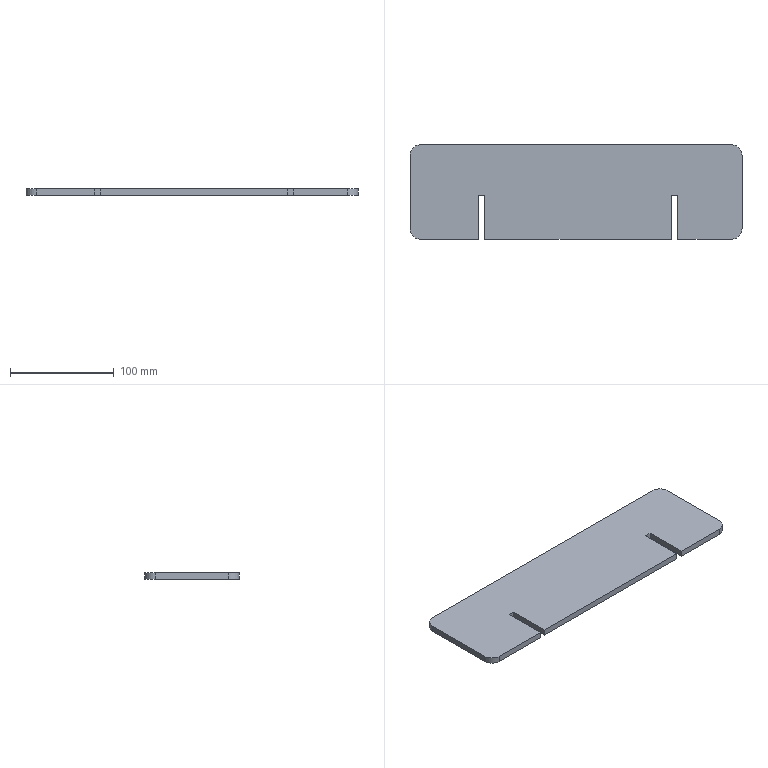Part | SolidWorks | features Fillet 1, FlatPattern 1, SMBaseFlange 1, SheetMetal 1 | 1 solid | 18 faces | box 320 x 91 x 6 mm | volume 171145 mm3 | plane 14 | cylinder 4 | commonest cylinder face diameters 20 x4
STEP:
#1=CARTESIAN_POINT('',(230.29,-583.5,-6.));
#2=VERTEX_POINT('',#1);
#3=CARTESIAN_POINT('',(230.29,-512.5,-6.));
#4=VERTEX_POINT('',#3);
#5=CARTESIAN_POINT('',(230.29,-502.5,-6.));
#6=DIRECTION('',(0.,1.,0.));
#7=VECTOR('',#6,1000.);
#8=LINE('',#5,#7);
#9=EDGE_CURVE('',#2,#4,#8,.T.);
#10=ORIENTED_EDGE('',*,*,#9,.T.);
#11=CARTESIAN_POINT('',(230.29,-512.5,0.));
#12=VERTEX_POINT('',#11);
#13=CARTESIAN_POINT('',(230.29,-512.5,-6.));
#14=DIRECTION('',(0.,0.,1.));
#15=VECTOR('',#14,1000.);
#16=LINE('',#13,#15);
#17=EDGE_CURVE('',#4,#12,#16,.T.);
#18=ORIENTED_EDGE('',*,*,#17,.T.);
#19=CARTESIAN_POINT('',(230.29,-583.5,0.));
#20=VERTEX_POINT('',#19);
#21=CARTESIAN_POINT('',(230.29,-502.5,0.));
#22=DIRECTION('',(0.,1.,0.));
#23=VECTOR('',#22,1000.);
#24=LINE('',#21,#23);
#25=EDGE_CURVE('',#20,#12,#24,.T.);
#26=ORIENTED_EDGE('',*,*,#25,.F.);
#27=CARTESIAN_POINT('',(230.29,-583.5,-6.));
#28=DIRECTION('',(0.,0.,1.));
#29=VECTOR('',#28,1000.);
#30=LINE('',#27,#29);
#31=EDGE_CURVE('',#2,#20,#30,.T.);
#32=ORIENTED_EDGE('',*,*,#31,.F.);
#33=EDGE_LOOP('',(#10,#18,#26,#32));
#34=FACE_OUTER_BOUND('',#33,.T.);
#35=CARTESIAN_POINT('',(230.29,-502.5,-6.));
#36=DIRECTION('',(1.,0.,0.));
#37=DIRECTION('',(0.,1.,0.));
#38=AXIS2_PLACEMENT_3D('',#35,#36,#37);
#39=PLANE('',#38);
#40=ADVANCED_FACE('',(#34),#39,.T.);
#41=CARTESIAN_POINT('',(220.29,-593.5,0.));
#42=VERTEX_POINT('',#41);
#43=CARTESIAN_POINT('',(220.29,-583.5,0.));
#44=DIRECTION('',(0.,0.,1.));
#45=DIRECTION('',(-1.,0.,0.));
#46=AXIS2_PLACEMENT_3D('',#43,#44,#45);
#47=CIRCLE('',#46,10.);
#48=EDGE_CURVE('',#42,#20,#47,.T.);
#49=ORIENTED_EDGE('',*,*,#48,.F.);
#50=CARTESIAN_POINT('',(220.29,-593.5,-6.));
#51=VERTEX_POINT('',#50);
#52=CARTESIAN_POINT('',(220.29,-593.5,-6.));
#53=DIRECTION('',(0.,0.,1.));
#54=VECTOR('',#53,1000.);
#55=LINE('',#52,#54);
#56=EDGE_CURVE('',#51,#42,#55,.T.);
#57=ORIENTED_EDGE('',*,*,#56,.F.);
#58=CARTESIAN_POINT('',(220.29,-583.5,-6.));
#59=DIRECTION('',(0.,0.,1.));
#60=DIRECTION('',(-1.,0.,0.));
#61=AXIS2_PLACEMENT_3D('',#58,#59,#60);
#62=CIRCLE('',#61,10.);
#63=EDGE_CURVE('',#51,#2,#62,.T.);
#64=ORIENTED_EDGE('',*,*,#63,.T.);
#65=ORIENTED_EDGE('',*,*,#31,.T.);
#66=EDGE_LOOP('',(#49,#57,#64,#65));
#67=FACE_OUTER_BOUND('',#66,.T.);
#68=CARTESIAN_POINT('',(220.29,-583.5,-6.));
#69=DIRECTION('',(0.,0.,1.));
#70=DIRECTION('',(1.,0.,0.));
#71=AXIS2_PLACEMENT_3D('',#68,#69,#70);
#72=CYLINDRICAL_SURFACE('',#71,10.);
#73=ADVANCED_FACE('',(#67),#72,.T.);
#74=CARTESIAN_POINT('',(168.29,-593.5,0.));
#75=VERTEX_POINT('',#74);
#76=CARTESIAN_POINT('',(220.29,-593.5,0.));
#77=DIRECTION('',(1.,0.,0.));
#78=VECTOR('',#77,1000.);
#79=LINE('',#76,#78);
#80=EDGE_CURVE('',#75,#42,#79,.T.);
#81=ORIENTED_EDGE('',*,*,#80,.F.);
#82=CARTESIAN_POINT('',(168.29,-593.5,-6.));
#83=VERTEX_POINT('',#82);
#84=CARTESIAN_POINT('',(168.29,-593.5,-6.));
#85=DIRECTION('',(0.,0.,1.));
#86=VECTOR('',#85,1000.);
#87=LINE('',#84,#86);
#88=EDGE_CURVE('',#83,#75,#87,.T.);
#89=ORIENTED_EDGE('',*,*,#88,.F.);
#90=CARTESIAN_POINT('',(220.29,-593.5,-6.));
#91=DIRECTION('',(1.,0.,0.));
#92=VECTOR('',#91,1000.);
#93=LINE('',#90,#92);
#94=EDGE_CURVE('',#83,#51,#93,.T.);
#95=ORIENTED_EDGE('',*,*,#94,.T.);
#96=ORIENTED_EDGE('',*,*,#56,.T.);
#97=EDGE_LOOP('',(#81,#89,#95,#96));
#98=FACE_OUTER_BOUND('',#97,.T.);
#99=CARTESIAN_POINT('',(220.29,-593.5,-6.));
#100=DIRECTION('',(0.,-1.,0.));
#101=DIRECTION('',(0.,0.,-1.));
#102=AXIS2_PLACEMENT_3D('',#99,#100,#101);
#103=PLANE('',#102);
#104=ADVANCED_FACE('',(#98),#103,.T.);
#105=CARTESIAN_POINT('',(168.29,-551.,0.));
#106=VERTEX_POINT('',#105);
#107=CARTESIAN_POINT('',(168.29,-593.5,0.));
#108=DIRECTION('',(0.,-1.,0.));
#109=VECTOR('',#108,1000.);
#110=LINE('',#107,#109);
#111=EDGE_CURVE('',#106,#75,#110,.T.);
#112=ORIENTED_EDGE('',*,*,#111,.F.);
#113=CARTESIAN_POINT('',(168.29,-551.,-6.));
#114=VERTEX_POINT('',#113);
#115=CARTESIAN_POINT('',(168.29,-551.,-6.));
#116=DIRECTION('',(0.,0.,1.));
#117=VECTOR('',#116,1000.);
#118=LINE('',#115,#117);
#119=EDGE_CURVE('',#114,#106,#118,.T.);
#120=ORIENTED_EDGE('',*,*,#119,.F.);
#121=CARTESIAN_POINT('',(168.29,-593.5,-6.));
#122=DIRECTION('',(0.,-1.,0.));
#123=VECTOR('',#122,1000.);
#124=LINE('',#121,#123);
#125=EDGE_CURVE('',#114,#83,#124,.T.);
#126=ORIENTED_EDGE('',*,*,#125,.T.);
#127=ORIENTED_EDGE('',*,*,#88,.T.);
#128=EDGE_LOOP('',(#112,#120,#126,#127));
#129=FACE_OUTER_BOUND('',#128,.T.);
#130=CARTESIAN_POINT('',(168.29,-593.5,-6.));
#131=DIRECTION('',(-1.,0.,0.));
#132=DIRECTION('',(0.,0.,1.));
#133=AXIS2_PLACEMENT_3D('',#130,#131,#132);
#134=PLANE('',#133);
#135=ADVANCED_FACE('',(#129),#134,.T.);
#136=CARTESIAN_POINT('',(162.29,-551.,0.));
#137=VERTEX_POINT('',#136);
#138=CARTESIAN_POINT('',(168.29,-551.,0.));
#139=DIRECTION('',(1.,0.,0.));
#140=VECTOR('',#139,1000.);
#141=LINE('',#138,#140);
#142=EDGE_CURVE('',#137,#106,#141,.T.);
#143=ORIENTED_EDGE('',*,*,#142,.F.);
#144=CARTESIAN_POINT('',(162.29,-551.,-6.));
#145=VERTEX_POINT('',#144);
#146=CARTESIAN_POINT('',(162.29,-551.,-6.));
#147=DIRECTION('',(0.,0.,1.));
#148=VECTOR('',#147,1000.);
#149=LINE('',#146,#148);
#150=EDGE_CURVE('',#145,#137,#149,.T.);
#151=ORIENTED_EDGE('',*,*,#150,.F.);
#152=CARTESIAN_POINT('',(168.29,-551.,-6.));
#153=DIRECTION('',(1.,0.,0.));
#154=VECTOR('',#153,1000.);
#155=LINE('',#152,#154);
#156=EDGE_CURVE('',#145,#114,#155,.T.);
#157=ORIENTED_EDGE('',*,*,#156,.T.);
#158=ORIENTED_EDGE('',*,*,#119,.T.);
#159=EDGE_LOOP('',(#143,#151,#157,#158));
#160=FACE_OUTER_BOUND('',#159,.T.);
#161=CARTESIAN_POINT('',(168.29,-551.,-6.));
#162=DIRECTION('',(0.,-1.,0.));
#163=DIRECTION('',(0.,0.,-1.));
#164=AXIS2_PLACEMENT_3D('',#161,#162,#163);
#165=PLANE('',#164);
#166=ADVANCED_FACE('',(#160),#165,.T.);
#167=CARTESIAN_POINT('',(162.29,-593.5,0.));
#168=VERTEX_POINT('',#167);
#169=CARTESIAN_POINT('',(162.29,-551.,0.));
#170=DIRECTION('',(0.,1.,0.));
#171=VECTOR('',#170,1000.);
#172=LINE('',#169,#171);
#173=EDGE_CURVE('',#168,#137,#172,.T.);
#174=ORIENTED_EDGE('',*,*,#173,.F.);
#175=CARTESIAN_POINT('',(162.29,-593.5,-6.));
#176=VERTEX_POINT('',#175);
#177=CARTESIAN_POINT('',(162.29,-593.5,-6.));
#178=DIRECTION('',(0.,0.,1.));
#179=VECTOR('',#178,1000.);
#180=LINE('',#177,#179);
#181=EDGE_CURVE('',#176,#168,#180,.T.);
#182=ORIENTED_EDGE('',*,*,#181,.F.);
#183=CARTESIAN_POINT('',(162.29,-551.,-6.));
#184=DIRECTION('',(0.,1.,0.));
#185=VECTOR('',#184,1000.);
#186=LINE('',#183,#185);
#187=EDGE_CURVE('',#176,#145,#186,.T.);
#188=ORIENTED_EDGE('',*,*,#187,.T.);
#189=ORIENTED_EDGE('',*,*,#150,.T.);
#190=EDGE_LOOP('',(#174,#182,#188,#189));
#191=FACE_OUTER_BOUND('',#190,.T.);
#192=CARTESIAN_POINT('',(162.29,-551.,-6.));
#193=DIRECTION('',(1.,0.,0.));
#194=DIRECTION('',(0.,1.,0.));
#195=AXIS2_PLACEMENT_3D('',#192,#193,#194);
#196=PLANE('',#195);
#197=ADVANCED_FACE('',(#191),#196,.T.);
#198=CARTESIAN_POINT('',(-17.71,-593.5,0.));
#199=VERTEX_POINT('',#198);
#200=CARTESIAN_POINT('',(162.29,-593.5,0.));
#201=DIRECTION('',(1.,0.,0.));
#202=VECTOR('',#201,1000.);
#203=LINE('',#200,#202);
#204=EDGE_CURVE('',#199,#168,#203,.T.);
#205=ORIENTED_EDGE('',*,*,#204,.F.);
#206=CARTESIAN_POINT('',(-17.71,-593.5,-6.));
#207=VERTEX_POINT('',#206);
#208=CARTESIAN_POINT('',(-17.71,-593.5,-6.));
#209=DIRECTION('',(0.,0.,1.));
#210=VECTOR('',#209,1000.);
#211=LINE('',#208,#210);
#212=EDGE_CURVE('',#207,#199,#211,.T.);
#213=ORIENTED_EDGE('',*,*,#212,.F.);
#214=CARTESIAN_POINT('',(162.29,-593.5,-6.));
#215=DIRECTION('',(1.,0.,0.));
#216=VECTOR('',#215,1000.);
#217=LINE('',#214,#216);
#218=EDGE_CURVE('',#207,#176,#217,.T.);
#219=ORIENTED_EDGE('',*,*,#218,.T.);
#220=ORIENTED_EDGE('',*,*,#181,.T.);
#221=EDGE_LOOP('',(#205,#213,#219,#220));
#222=FACE_OUTER_BOUND('',#221,.T.);
#223=CARTESIAN_POINT('',(162.29,-593.5,-6.));
#224=DIRECTION('',(0.,-1.,0.));
#225=DIRECTION('',(0.,0.,-1.));
#226=AXIS2_PLACEMENT_3D('',#223,#224,#225);
#227=PLANE('',#226);
#228=ADVANCED_FACE('',(#222),#227,.T.);
#229=CARTESIAN_POINT('',(-17.71,-551.,0.));
#230=VERTEX_POINT('',#229);
#231=CARTESIAN_POINT('',(-17.71,-593.5,0.));
#232=DIRECTION('',(0.,-1.,0.));
#233=VECTOR('',#232,1000.);
#234=LINE('',#231,#233);
#235=EDGE_CURVE('',#230,#199,#234,.T.);
#236=ORIENTED_EDGE('',*,*,#235,.F.);
#237=CARTESIAN_POINT('',(-17.71,-551.,-6.));
#238=VERTEX_POINT('',#237);
#239=CARTESIAN_POINT('',(-17.71,-551.,-6.));
#240=DIRECTION('',(0.,0.,1.));
#241=VECTOR('',#240,1000.);
#242=LINE('',#239,#241);
#243=EDGE_CURVE('',#238,#230,#242,.T.);
#244=ORIENTED_EDGE('',*,*,#243,.F.);
#245=CARTESIAN_POINT('',(-17.71,-593.5,-6.));
#246=DIRECTION('',(0.,-1.,0.));
#247=VECTOR('',#246,1000.);
#248=LINE('',#245,#247);
#249=EDGE_CURVE('',#238,#207,#248,.T.);
#250=ORIENTED_EDGE('',*,*,#249,.T.);
#251=ORIENTED_EDGE('',*,*,#212,.T.);
#252=EDGE_LOOP('',(#236,#244,#250,#251));
#253=FACE_OUTER_BOUND('',#252,.T.);
#254=CARTESIAN_POINT('',(-17.71,-593.5,-6.));
#255=DIRECTION('',(-1.,0.,0.));
#256=DIRECTION('',(0.,-1.,0.));
#257=AXIS2_PLACEMENT_3D('',#254,#255,#256);
#258=PLANE('',#257);
#259=ADVANCED_FACE('',(#253),#258,.T.);
#260=CARTESIAN_POINT('',(-23.71,-551.,0.));
#261=VERTEX_POINT('',#260);
#262=CARTESIAN_POINT('',(-17.71,-551.,0.));
#263=DIRECTION('',(1.,0.,0.));
#264=VECTOR('',#263,1000.);
#265=LINE('',#262,#264);
#266=EDGE_CURVE('',#261,#230,#265,.T.);
#267=ORIENTED_EDGE('',*,*,#266,.F.);
#268=CARTESIAN_POINT('',(-23.71,-551.,-6.));
#269=VERTEX_POINT('',#268);
#270=CARTESIAN_POINT('',(-23.71,-551.,-6.));
#271=DIRECTION('',(0.,0.,1.));
#272=VECTOR('',#271,1000.);
#273=LINE('',#270,#272);
#274=EDGE_CURVE('',#269,#261,#273,.T.);
#275=ORIENTED_EDGE('',*,*,#274,.F.);
#276=CARTESIAN_POINT('',(-17.71,-551.,-6.));
#277=DIRECTION('',(1.,0.,0.));
#278=VECTOR('',#277,1000.);
#279=LINE('',#276,#278);
#280=EDGE_CURVE('',#269,#238,#279,.T.);
#281=ORIENTED_EDGE('',*,*,#280,.T.);
#282=ORIENTED_EDGE('',*,*,#243,.T.);
#283=EDGE_LOOP('',(#267,#275,#281,#282));
#284=FACE_OUTER_BOUND('',#283,.T.);
#285=CARTESIAN_POINT('',(-17.71,-551.,-6.));
#286=DIRECTION('',(0.,-1.,0.));
#287=DIRECTION('',(0.,0.,-1.));
#288=AXIS2_PLACEMENT_3D('',#285,#286,#287);
#289=PLANE('',#288);
#290=ADVANCED_FACE('',(#284),#289,.T.);
#291=CARTESIAN_POINT('',(-23.71,-593.5,0.));
#292=VERTEX_POINT('',#291);
#293=CARTESIAN_POINT('',(-23.71,-551.,0.));
#294=DIRECTION('',(0.,1.,0.));
#295=VECTOR('',#294,1000.);
#296=LINE('',#293,#295);
#297=EDGE_CURVE('',#292,#261,#296,.T.);
#298=ORIENTED_EDGE('',*,*,#297,.F.);
#299=CARTESIAN_POINT('',(-23.71,-593.5,-6.));
#300=VERTEX_POINT('',#299);
#301=CARTESIAN_POINT('',(-23.71,-593.5,-6.));
#302=DIRECTION('',(0.,0.,1.));
#303=VECTOR('',#302,1000.);
#304=LINE('',#301,#303);
#305=EDGE_CURVE('',#300,#292,#304,.T.);
#306=ORIENTED_EDGE('',*,*,#305,.F.);
#307=CARTESIAN_POINT('',(-23.71,-551.,-6.));
#308=DIRECTION('',(0.,1.,0.));
#309=VECTOR('',#308,1000.);
#310=LINE('',#307,#309);
#311=EDGE_CURVE('',#300,#269,#310,.T.);
#312=ORIENTED_EDGE('',*,*,#311,.T.);
#313=ORIENTED_EDGE('',*,*,#274,.T.);
#314=EDGE_LOOP('',(#298,#306,#312,#313));
#315=FACE_OUTER_BOUND('',#314,.T.);
#316=CARTESIAN_POINT('',(-23.71,-551.,-6.));
#317=DIRECTION('',(1.,0.,0.));
#318=DIRECTION('',(0.,1.,0.));
#319=AXIS2_PLACEMENT_3D('',#316,#317,#318);
#320=PLANE('',#319);
#321=ADVANCED_FACE('',(#315),#320,.T.);
#322=CARTESIAN_POINT('',(-79.71,-593.5,0.));
#323=VERTEX_POINT('',#322);
#324=CARTESIAN_POINT('',(-23.71,-593.5,0.));
#325=DIRECTION('',(1.,0.,0.));
#326=VECTOR('',#325,1000.);
#327=LINE('',#324,#326);
#328=EDGE_CURVE('',#323,#292,#327,.T.);
#329=ORIENTED_EDGE('',*,*,#328,.F.);
#330=CARTESIAN_POINT('',(-79.71,-593.5,-6.));
#331=VERTEX_POINT('',#330);
#332=CARTESIAN_POINT('',(-79.71,-593.5,-6.));
#333=DIRECTION('',(0.,0.,1.));
#334=VECTOR('',#333,1000.);
#335=LINE('',#332,#334);
#336=EDGE_CURVE('',#331,#323,#335,.T.);
#337=ORIENTED_EDGE('',*,*,#336,.F.);
#338=CARTESIAN_POINT('',(-23.71,-593.5,-6.));
#339=DIRECTION('',(1.,0.,0.));
#340=VECTOR('',#339,1000.);
#341=LINE('',#338,#340);
#342=EDGE_CURVE('',#331,#300,#341,.T.);
#343=ORIENTED_EDGE('',*,*,#342,.T.);
#344=ORIENTED_EDGE('',*,*,#305,.T.);
#345=EDGE_LOOP('',(#329,#337,#343,#344));
#346=FACE_OUTER_BOUND('',#345,.T.);
#347=CARTESIAN_POINT('',(-23.71,-593.5,-6.));
#348=DIRECTION('',(0.,-1.,0.));
#349=DIRECTION('',(0.,0.,-1.));
#350=AXIS2_PLACEMENT_3D('',#347,#348,#349);
#351=PLANE('',#350);
#352=ADVANCED_FACE('',(#346),#351,.T.);
#353=CARTESIAN_POINT('',(-89.71,-583.5,0.));
#354=VERTEX_POINT('',#353);
#355=CARTESIAN_POINT('',(-79.71,-583.5,0.));
#356=DIRECTION('',(0.,0.,1.));
#357=DIRECTION('',(-1.,0.,0.));
#358=AXIS2_PLACEMENT_3D('',#355,#356,#357);
#359=CIRCLE('',#358,10.);
#360=EDGE_CURVE('',#354,#323,#359,.T.);
#361=ORIENTED_EDGE('',*,*,#360,.F.);
#362=CARTESIAN_POINT('',(-89.71,-583.5,-6.));
#363=VERTEX_POINT('',#362);
#364=CARTESIAN_POINT('',(-89.71,-583.5,-6.));
#365=DIRECTION('',(0.,0.,1.));
#366=VECTOR('',#365,1000.);
#367=LINE('',#364,#366);
#368=EDGE_CURVE('',#363,#354,#367,.T.);
#369=ORIENTED_EDGE('',*,*,#368,.F.);
#370=CARTESIAN_POINT('',(-79.71,-583.5,-6.));
#371=DIRECTION('',(0.,0.,1.));
#372=DIRECTION('',(-1.,0.,0.));
#373=AXIS2_PLACEMENT_3D('',#370,#371,#372);
#374=CIRCLE('',#373,10.);
#375=EDGE_CURVE('',#363,#331,#374,.T.);
#376=ORIENTED_EDGE('',*,*,#375,.T.);
#377=ORIENTED_EDGE('',*,*,#336,.T.);
#378=EDGE_LOOP('',(#361,#369,#376,#377));
#379=FACE_OUTER_BOUND('',#378,.T.);
#380=CARTESIAN_POINT('',(-79.71,-583.5,-6.));
#381=DIRECTION('',(0.,0.,1.));
#382=DIRECTION('',(1.,0.,0.));
#383=AXIS2_PLACEMENT_3D('',#380,#381,#382);
#384=CYLINDRICAL_SURFACE('',#383,10.);
#385=ADVANCED_FACE('',(#379),#384,.T.);
#386=CARTESIAN_POINT('',(-89.71,-512.5,0.));
#387=VERTEX_POINT('',#386);
#388=CARTESIAN_POINT('',(-89.71,-502.5,0.));
#389=DIRECTION('',(0.,-1.,0.));
#390=VECTOR('',#389,1000.);
#391=LINE('',#388,#390);
#392=EDGE_CURVE('',#387,#354,#391,.T.);
#393=ORIENTED_EDGE('',*,*,#392,.F.);
#394=CARTESIAN_POINT('',(-89.71,-512.5,-6.));
#395=VERTEX_POINT('',#394);
#396=CARTESIAN_POINT('',(-89.71,-512.5,-6.));
#397=DIRECTION('',(0.,0.,-1.));
#398=VECTOR('',#397,1000.);
#399=LINE('',#396,#398);
#400=EDGE_CURVE('',#387,#395,#399,.T.);
#401=ORIENTED_EDGE('',*,*,#400,.T.);
#402=CARTESIAN_POINT('',(-89.71,-502.5,-6.));
#403=DIRECTION('',(0.,-1.,0.));
#404=VECTOR('',#403,1000.);
#405=LINE('',#402,#404);
#406=EDGE_CURVE('',#395,#363,#405,.T.);
#407=ORIENTED_EDGE('',*,*,#406,.T.);
#408=ORIENTED_EDGE('',*,*,#368,.T.);
#409=EDGE_LOOP('',(#393,#401,#407,#408));
#410=FACE_OUTER_BOUND('',#409,.T.);
#411=CARTESIAN_POINT('',(-89.71,-502.5,-6.));
#412=DIRECTION('',(-1.,0.,0.));
#413=DIRECTION('',(0.,-1.,0.));
#414=AXIS2_PLACEMENT_3D('',#411,#412,#413);
#415=PLANE('',#414);
#416=ADVANCED_FACE('',(#410),#415,.T.);
#417=CARTESIAN_POINT('',(220.29,-502.5,0.));
#418=VERTEX_POINT('',#417);
#419=CARTESIAN_POINT('',(-79.71,-502.5,0.));
#420=VERTEX_POINT('',#419);
#421=CARTESIAN_POINT('',(230.29,-502.5,0.));
#422=DIRECTION('',(-1.,0.,0.));
#423=VECTOR('',#422,1000.);
#424=LINE('',#421,#423);
#425=EDGE_CURVE('',#418,#420,#424,.T.);
#426=ORIENTED_EDGE('',*,*,#425,.F.);
#427=CARTESIAN_POINT('',(220.29,-502.5,-6.));
#428=VERTEX_POINT('',#427);
#429=CARTESIAN_POINT('',(220.29,-502.5,-6.));
#430=DIRECTION('',(0.,0.,-1.));
#431=VECTOR('',#430,1000.);
#432=LINE('',#429,#431);
#433=EDGE_CURVE('',#418,#428,#432,.T.);
#434=ORIENTED_EDGE('',*,*,#433,.T.);
#435=CARTESIAN_POINT('',(-79.71,-502.5,-6.));
#436=VERTEX_POINT('',#435);
#437=CARTESIAN_POINT('',(230.29,-502.5,-6.));
#438=DIRECTION('',(-1.,0.,0.));
#439=VECTOR('',#438,1000.);
#440=LINE('',#437,#439);
#441=EDGE_CURVE('',#428,#436,#440,.T.);
#442=ORIENTED_EDGE('',*,*,#441,.T.);
#443=CARTESIAN_POINT('',(-79.71,-502.5,-6.));
#444=DIRECTION('',(0.,0.,1.));
#445=VECTOR('',#444,1000.);
#446=LINE('',#443,#445);
#447=EDGE_CURVE('',#436,#420,#446,.T.);
#448=ORIENTED_EDGE('',*,*,#447,.T.);
#449=EDGE_LOOP('',(#426,#434,#442,#448));
#450=FACE_OUTER_BOUND('',#449,.T.);
#451=CARTESIAN_POINT('',(230.29,-502.5,-6.));
#452=DIRECTION('',(0.,1.,0.));
#453=DIRECTION('',(0.,0.,1.));
#454=AXIS2_PLACEMENT_3D('',#451,#452,#453);
#455=PLANE('',#454);
#456=ADVANCED_FACE('',(#450),#455,.T.);
#457=ORIENTED_EDGE('',*,*,#441,.F.);
#458=CARTESIAN_POINT('',(220.29,-512.5,-6.));
#459=DIRECTION('',(0.,0.,-1.));
#460=DIRECTION('',(-1.,0.,0.));
#461=AXIS2_PLACEMENT_3D('',#458,#459,#460);
#462=CIRCLE('',#461,10.);
#463=EDGE_CURVE('',#428,#4,#462,.T.);
#464=ORIENTED_EDGE('',*,*,#463,.T.);
#465=ORIENTED_EDGE('',*,*,#9,.F.);
#466=ORIENTED_EDGE('',*,*,#63,.F.);
#467=ORIENTED_EDGE('',*,*,#94,.F.);
#468=ORIENTED_EDGE('',*,*,#125,.F.);
#469=ORIENTED_EDGE('',*,*,#156,.F.);
#470=ORIENTED_EDGE('',*,*,#187,.F.);
#471=ORIENTED_EDGE('',*,*,#218,.F.);
#472=ORIENTED_EDGE('',*,*,#249,.F.);
#473=ORIENTED_EDGE('',*,*,#280,.F.);
#474=ORIENTED_EDGE('',*,*,#311,.F.);
#475=ORIENTED_EDGE('',*,*,#342,.F.);
#476=ORIENTED_EDGE('',*,*,#375,.F.);
#477=ORIENTED_EDGE('',*,*,#406,.F.);
#478=CARTESIAN_POINT('',(-79.71,-512.5,-6.));
#479=DIRECTION('',(0.,0.,-1.));
#480=DIRECTION('',(-1.,0.,0.));
#481=AXIS2_PLACEMENT_3D('',#478,#479,#480);
#482=CIRCLE('',#481,10.);
#483=EDGE_CURVE('',#395,#436,#482,.T.);
#484=ORIENTED_EDGE('',*,*,#483,.T.);
#485=EDGE_LOOP('',(#457,#464,#465,#466,#467,#468,#469,#470,#471,#472,#473,#474,#475,#476,#477,#484));
#486=FACE_OUTER_BOUND('',#485,.T.);
#487=CARTESIAN_POINT('',(220.29,-583.5,-6.));
#488=DIRECTION('',(0.,0.,-1.));
#489=DIRECTION('',(-1.,0.,0.));
#490=AXIS2_PLACEMENT_3D('',#487,#488,#489);
#491=PLANE('',#490);
#492=ADVANCED_FACE('',(#486),#491,.T.);
#493=ORIENTED_EDGE('',*,*,#25,.T.);
#494=CARTESIAN_POINT('',(220.29,-512.5,0.));
#495=DIRECTION('',(0.,0.,1.));
#496=DIRECTION('',(-1.,0.,0.));
#497=AXIS2_PLACEMENT_3D('',#494,#495,#496);
#498=CIRCLE('',#497,10.);
#499=EDGE_CURVE('',#12,#418,#498,.T.);
#500=ORIENTED_EDGE('',*,*,#499,.T.);
#501=ORIENTED_EDGE('',*,*,#425,.T.);
#502=CARTESIAN_POINT('',(-79.71,-512.5,0.));
#503=DIRECTION('',(0.,0.,1.));
#504=DIRECTION('',(-1.,0.,0.));
#505=AXIS2_PLACEMENT_3D('',#502,#503,#504);
#506=CIRCLE('',#505,10.);
#507=EDGE_CURVE('',#420,#387,#506,.T.);
#508=ORIENTED_EDGE('',*,*,#507,.T.);
#509=ORIENTED_EDGE('',*,*,#392,.T.);
#510=ORIENTED_EDGE('',*,*,#360,.T.);
#511=ORIENTED_EDGE('',*,*,#328,.T.);
#512=ORIENTED_EDGE('',*,*,#297,.T.);
#513=ORIENTED_EDGE('',*,*,#266,.T.);
#514=ORIENTED_EDGE('',*,*,#235,.T.);
#515=ORIENTED_EDGE('',*,*,#204,.T.);
#516=ORIENTED_EDGE('',*,*,#173,.T.);
#517=ORIENTED_EDGE('',*,*,#142,.T.);
#518=ORIENTED_EDGE('',*,*,#111,.T.);
#519=ORIENTED_EDGE('',*,*,#80,.T.);
#520=ORIENTED_EDGE('',*,*,#48,.T.);
#521=EDGE_LOOP('',(#493,#500,#501,#508,#509,#510,#511,#512,#513,#514,#515,#516,#517,#518,#519,#520));
#522=FACE_OUTER_BOUND('',#521,.T.);
#523=CARTESIAN_POINT('',(220.29,-583.5,0.));
#524=DIRECTION('',(0.,0.,-1.));
#525=DIRECTION('',(-1.,0.,0.));
#526=AXIS2_PLACEMENT_3D('',#523,#524,#525);
#527=PLANE('',#526);
#528=ADVANCED_FACE('',(#522),#527,.F.);
#529=ORIENTED_EDGE('',*,*,#463,.F.);
#530=ORIENTED_EDGE('',*,*,#433,.F.);
#531=ORIENTED_EDGE('',*,*,#499,.F.);
#532=ORIENTED_EDGE('',*,*,#17,.F.);
#533=EDGE_LOOP('',(#529,#530,#531,#532));
#534=FACE_OUTER_BOUND('',#533,.T.);
#535=CARTESIAN_POINT('',(220.29,-512.5,-6.));
#536=DIRECTION('',(0.,0.,1.));
#537=DIRECTION('',(1.,0.,0.));
#538=AXIS2_PLACEMENT_3D('',#535,#536,#537);
#539=CYLINDRICAL_SURFACE('',#538,10.);
#540=ADVANCED_FACE('',(#534),#539,.T.);
#541=ORIENTED_EDGE('',*,*,#483,.F.);
#542=ORIENTED_EDGE('',*,*,#400,.F.);
#543=ORIENTED_EDGE('',*,*,#507,.F.);
#544=ORIENTED_EDGE('',*,*,#447,.F.);
#545=EDGE_LOOP('',(#541,#542,#543,#544));
#546=FACE_OUTER_BOUND('',#545,.T.);
#547=CARTESIAN_POINT('',(-79.71,-512.5,-6.));
#548=DIRECTION('',(0.,0.,1.));
#549=DIRECTION('',(1.,0.,0.));
#550=AXIS2_PLACEMENT_3D('',#547,#548,#549);
#551=CYLINDRICAL_SURFACE('',#550,10.);
#552=ADVANCED_FACE('',(#546),#551,.T.);
#553=CLOSED_SHELL('',(#40,#73,#104,#135,#166,#197,#228,#259,#290,#321,#352,#385,#416,#456,#492,#528,#540,#552));
#554=MANIFOLD_SOLID_BREP('',#553);
#555=CARTESIAN_POINT('',(0.,0.,0.));
#556=DIRECTION('',(0.,0.,1.));
#557=DIRECTION('',(1.,0.,0.));
#558=AXIS2_PLACEMENT_3D('',#555,#556,#557);
#559=(LENGTH_UNIT()NAMED_UNIT(*)SI_UNIT(.MILLI.,.METRE.));
#560=UNCERTAINTY_MEASURE_WITH_UNIT(LENGTH_MEASURE(0.00001),#559,'','');
#561=(NAMED_UNIT(*)PLANE_ANGLE_UNIT()SI_UNIT($,.RADIAN.));
#562=(NAMED_UNIT(*)SI_UNIT($,.STERADIAN.)SOLID_ANGLE_UNIT());
#563=(GEOMETRIC_REPRESENTATION_CONTEXT(3)GLOBAL_UNCERTAINTY_ASSIGNED_CONTEXT((#560))GLOBAL_UNIT_ASSIGNED_CONTEXT((#559,#561,#562))REPRESENTATION_CONTEXT('',''));
#564=ADVANCED_BREP_SHAPE_REPRESENTATION('',(#554,#558),#563);